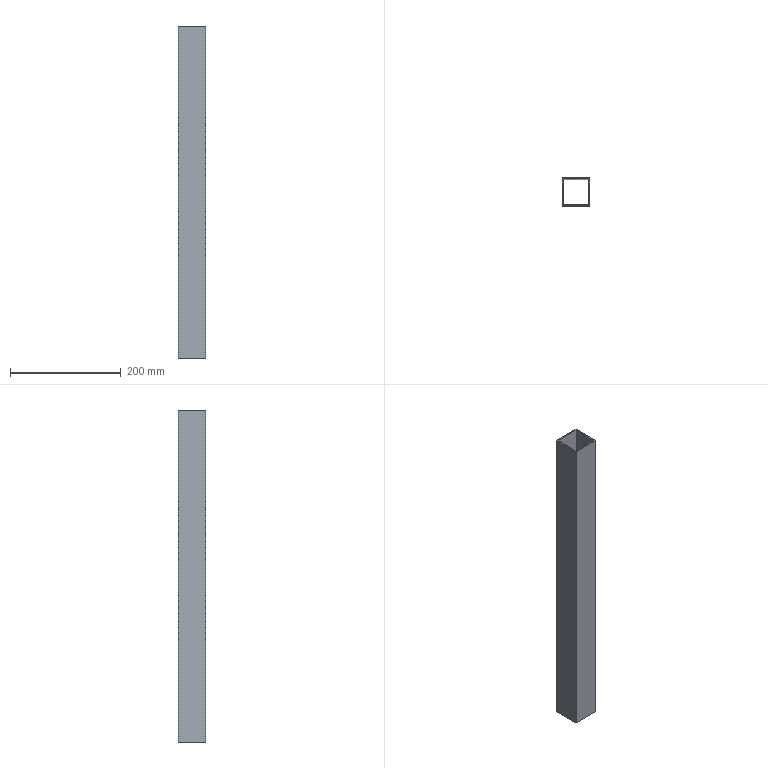Part | SolidWorks | features Extrusion 1 | 1 solid | 10 faces | box 50 x 50 x 600 mm | volume 230400 mm3 | plane 10
STEP:
#1=CARTESIAN_POINT('',(25.,-25.,600.));
#2=VERTEX_POINT('',#1);
#3=CARTESIAN_POINT('',(25.,25.,600.));
#4=VERTEX_POINT('',#3);
#5=CARTESIAN_POINT('',(25.,-25.,600.));
#6=DIRECTION('',(0.,1.,0.));
#7=VECTOR('',#6,1000.);
#8=LINE('',#5,#7);
#9=EDGE_CURVE('',#2,#4,#8,.T.);
#10=ORIENTED_EDGE('',*,*,#9,.T.);
#11=CARTESIAN_POINT('',(-25.,25.,600.));
#12=VERTEX_POINT('',#11);
#13=CARTESIAN_POINT('',(-25.,25.,600.));
#14=DIRECTION('',(-1.,0.,0.));
#15=VECTOR('',#14,1000.);
#16=LINE('',#13,#15);
#17=EDGE_CURVE('',#4,#12,#16,.T.);
#18=ORIENTED_EDGE('',*,*,#17,.T.);
#19=CARTESIAN_POINT('',(-25.,-25.,600.));
#20=VERTEX_POINT('',#19);
#21=CARTESIAN_POINT('',(-25.,-25.,600.));
#22=DIRECTION('',(0.,-1.,0.));
#23=VECTOR('',#22,1000.);
#24=LINE('',#21,#23);
#25=EDGE_CURVE('',#12,#20,#24,.T.);
#26=ORIENTED_EDGE('',*,*,#25,.T.);
#27=CARTESIAN_POINT('',(-25.,-25.,600.));
#28=DIRECTION('',(1.,0.,0.));
#29=VECTOR('',#28,1000.);
#30=LINE('',#27,#29);
#31=EDGE_CURVE('',#20,#2,#30,.T.);
#32=ORIENTED_EDGE('',*,*,#31,.T.);
#33=EDGE_LOOP('',(#10,#18,#26,#32));
#34=FACE_OUTER_BOUND('',#33,.T.);
#35=CARTESIAN_POINT('',(23.,-23.,600.));
#36=VERTEX_POINT('',#35);
#37=CARTESIAN_POINT('',(23.,23.,600.));
#38=VERTEX_POINT('',#37);
#39=CARTESIAN_POINT('',(23.,-23.,600.));
#40=DIRECTION('',(0.,1.,0.));
#41=VECTOR('',#40,1000.);
#42=LINE('',#39,#41);
#43=EDGE_CURVE('',#36,#38,#42,.T.);
#44=ORIENTED_EDGE('',*,*,#43,.F.);
#45=CARTESIAN_POINT('',(-23.,-23.,600.));
#46=VERTEX_POINT('',#45);
#47=CARTESIAN_POINT('',(-23.,-23.,600.));
#48=DIRECTION('',(1.,0.,0.));
#49=VECTOR('',#48,1000.);
#50=LINE('',#47,#49);
#51=EDGE_CURVE('',#46,#36,#50,.T.);
#52=ORIENTED_EDGE('',*,*,#51,.F.);
#53=CARTESIAN_POINT('',(-23.,23.,600.));
#54=VERTEX_POINT('',#53);
#55=CARTESIAN_POINT('',(-23.,-23.,600.));
#56=DIRECTION('',(0.,-1.,0.));
#57=VECTOR('',#56,1000.);
#58=LINE('',#55,#57);
#59=EDGE_CURVE('',#54,#46,#58,.T.);
#60=ORIENTED_EDGE('',*,*,#59,.F.);
#61=CARTESIAN_POINT('',(-23.,23.,600.));
#62=DIRECTION('',(-1.,0.,0.));
#63=VECTOR('',#62,1000.);
#64=LINE('',#61,#63);
#65=EDGE_CURVE('',#38,#54,#64,.T.);
#66=ORIENTED_EDGE('',*,*,#65,.F.);
#67=EDGE_LOOP('',(#44,#52,#60,#66));
#68=FACE_BOUND('',#67,.T.);
#69=CARTESIAN_POINT('',(0.,0.,600.));
#70=DIRECTION('',(0.,0.,-1.));
#71=DIRECTION('',(-1.,0.,0.));
#72=AXIS2_PLACEMENT_3D('',#69,#70,#71);
#73=PLANE('',#72);
#74=ADVANCED_FACE('',(#34,#68),#73,.F.);
#75=CARTESIAN_POINT('',(25.,-25.,0.));
#76=VERTEX_POINT('',#75);
#77=CARTESIAN_POINT('',(25.,25.,0.));
#78=VERTEX_POINT('',#77);
#79=CARTESIAN_POINT('',(25.,-25.,0.));
#80=DIRECTION('',(0.,1.,0.));
#81=VECTOR('',#80,1000.);
#82=LINE('',#79,#81);
#83=EDGE_CURVE('',#76,#78,#82,.T.);
#84=ORIENTED_EDGE('',*,*,#83,.F.);
#85=CARTESIAN_POINT('',(-25.,-25.,0.));
#86=VERTEX_POINT('',#85);
#87=CARTESIAN_POINT('',(-25.,-25.,0.));
#88=DIRECTION('',(1.,0.,0.));
#89=VECTOR('',#88,1000.);
#90=LINE('',#87,#89);
#91=EDGE_CURVE('',#86,#76,#90,.T.);
#92=ORIENTED_EDGE('',*,*,#91,.F.);
#93=CARTESIAN_POINT('',(-25.,25.,0.));
#94=VERTEX_POINT('',#93);
#95=CARTESIAN_POINT('',(-25.,-25.,0.));
#96=DIRECTION('',(0.,-1.,0.));
#97=VECTOR('',#96,1000.);
#98=LINE('',#95,#97);
#99=EDGE_CURVE('',#94,#86,#98,.T.);
#100=ORIENTED_EDGE('',*,*,#99,.F.);
#101=CARTESIAN_POINT('',(-25.,25.,0.));
#102=DIRECTION('',(-1.,0.,0.));
#103=VECTOR('',#102,1000.);
#104=LINE('',#101,#103);
#105=EDGE_CURVE('',#78,#94,#104,.T.);
#106=ORIENTED_EDGE('',*,*,#105,.F.);
#107=EDGE_LOOP('',(#84,#92,#100,#106));
#108=FACE_OUTER_BOUND('',#107,.T.);
#109=CARTESIAN_POINT('',(-23.,-23.,0.));
#110=VERTEX_POINT('',#109);
#111=CARTESIAN_POINT('',(23.,-23.,0.));
#112=VERTEX_POINT('',#111);
#113=CARTESIAN_POINT('',(-23.,-23.,0.));
#114=DIRECTION('',(1.,0.,0.));
#115=VECTOR('',#114,1000.);
#116=LINE('',#113,#115);
#117=EDGE_CURVE('',#110,#112,#116,.T.);
#118=ORIENTED_EDGE('',*,*,#117,.T.);
#119=CARTESIAN_POINT('',(23.,23.,0.));
#120=VERTEX_POINT('',#119);
#121=CARTESIAN_POINT('',(23.,-23.,0.));
#122=DIRECTION('',(0.,1.,0.));
#123=VECTOR('',#122,1000.);
#124=LINE('',#121,#123);
#125=EDGE_CURVE('',#112,#120,#124,.T.);
#126=ORIENTED_EDGE('',*,*,#125,.T.);
#127=CARTESIAN_POINT('',(-23.,23.,0.));
#128=VERTEX_POINT('',#127);
#129=CARTESIAN_POINT('',(-23.,23.,0.));
#130=DIRECTION('',(-1.,0.,0.));
#131=VECTOR('',#130,1000.);
#132=LINE('',#129,#131);
#133=EDGE_CURVE('',#120,#128,#132,.T.);
#134=ORIENTED_EDGE('',*,*,#133,.T.);
#135=CARTESIAN_POINT('',(-23.,-23.,0.));
#136=DIRECTION('',(0.,-1.,0.));
#137=VECTOR('',#136,1000.);
#138=LINE('',#135,#137);
#139=EDGE_CURVE('',#128,#110,#138,.T.);
#140=ORIENTED_EDGE('',*,*,#139,.T.);
#141=EDGE_LOOP('',(#118,#126,#134,#140));
#142=FACE_BOUND('',#141,.T.);
#143=CARTESIAN_POINT('',(0.,0.,0.));
#144=DIRECTION('',(0.,0.,-1.));
#145=DIRECTION('',(-1.,0.,0.));
#146=AXIS2_PLACEMENT_3D('',#143,#144,#145);
#147=PLANE('',#146);
#148=ADVANCED_FACE('',(#108,#142),#147,.T.);
#149=ORIENTED_EDGE('',*,*,#83,.T.);
#150=CARTESIAN_POINT('',(25.,25.,600.));
#151=DIRECTION('',(0.,0.,-1.));
#152=VECTOR('',#151,1000.);
#153=LINE('',#150,#152);
#154=EDGE_CURVE('',#4,#78,#153,.T.);
#155=ORIENTED_EDGE('',*,*,#154,.F.);
#156=ORIENTED_EDGE('',*,*,#9,.F.);
#157=CARTESIAN_POINT('',(25.,-25.,600.));
#158=DIRECTION('',(0.,0.,-1.));
#159=VECTOR('',#158,1000.);
#160=LINE('',#157,#159);
#161=EDGE_CURVE('',#2,#76,#160,.T.);
#162=ORIENTED_EDGE('',*,*,#161,.T.);
#163=EDGE_LOOP('',(#149,#155,#156,#162));
#164=FACE_OUTER_BOUND('',#163,.T.);
#165=CARTESIAN_POINT('',(25.,-25.,600.));
#166=DIRECTION('',(-1.,0.,0.));
#167=DIRECTION('',(0.,0.,1.));
#168=AXIS2_PLACEMENT_3D('',#165,#166,#167);
#169=PLANE('',#168);
#170=ADVANCED_FACE('',(#164),#169,.F.);
#171=ORIENTED_EDGE('',*,*,#105,.T.);
#172=CARTESIAN_POINT('',(-25.,25.,600.));
#173=DIRECTION('',(0.,0.,-1.));
#174=VECTOR('',#173,1000.);
#175=LINE('',#172,#174);
#176=EDGE_CURVE('',#12,#94,#175,.T.);
#177=ORIENTED_EDGE('',*,*,#176,.F.);
#178=ORIENTED_EDGE('',*,*,#17,.F.);
#179=ORIENTED_EDGE('',*,*,#154,.T.);
#180=EDGE_LOOP('',(#171,#177,#178,#179));
#181=FACE_OUTER_BOUND('',#180,.T.);
#182=CARTESIAN_POINT('',(-25.,25.,600.));
#183=DIRECTION('',(0.,-1.,0.));
#184=DIRECTION('',(0.,0.,-1.));
#185=AXIS2_PLACEMENT_3D('',#182,#183,#184);
#186=PLANE('',#185);
#187=ADVANCED_FACE('',(#181),#186,.F.);
#188=ORIENTED_EDGE('',*,*,#99,.T.);
#189=CARTESIAN_POINT('',(-25.,-25.,600.));
#190=DIRECTION('',(0.,0.,-1.));
#191=VECTOR('',#190,1000.);
#192=LINE('',#189,#191);
#193=EDGE_CURVE('',#20,#86,#192,.T.);
#194=ORIENTED_EDGE('',*,*,#193,.F.);
#195=ORIENTED_EDGE('',*,*,#25,.F.);
#196=ORIENTED_EDGE('',*,*,#176,.T.);
#197=EDGE_LOOP('',(#188,#194,#195,#196));
#198=FACE_OUTER_BOUND('',#197,.T.);
#199=CARTESIAN_POINT('',(-25.,-25.,600.));
#200=DIRECTION('',(1.,0.,0.));
#201=DIRECTION('',(0.,0.,-1.));
#202=AXIS2_PLACEMENT_3D('',#199,#200,#201);
#203=PLANE('',#202);
#204=ADVANCED_FACE('',(#198),#203,.F.);
#205=ORIENTED_EDGE('',*,*,#91,.T.);
#206=ORIENTED_EDGE('',*,*,#161,.F.);
#207=ORIENTED_EDGE('',*,*,#31,.F.);
#208=ORIENTED_EDGE('',*,*,#193,.T.);
#209=EDGE_LOOP('',(#205,#206,#207,#208));
#210=FACE_OUTER_BOUND('',#209,.T.);
#211=CARTESIAN_POINT('',(-25.,-25.,600.));
#212=DIRECTION('',(0.,1.,0.));
#213=DIRECTION('',(0.,0.,1.));
#214=AXIS2_PLACEMENT_3D('',#211,#212,#213);
#215=PLANE('',#214);
#216=ADVANCED_FACE('',(#210),#215,.F.);
#217=ORIENTED_EDGE('',*,*,#125,.F.);
#218=CARTESIAN_POINT('',(23.,-23.,600.));
#219=DIRECTION('',(0.,0.,-1.));
#220=VECTOR('',#219,1000.);
#221=LINE('',#218,#220);
#222=EDGE_CURVE('',#36,#112,#221,.T.);
#223=ORIENTED_EDGE('',*,*,#222,.F.);
#224=ORIENTED_EDGE('',*,*,#43,.T.);
#225=CARTESIAN_POINT('',(23.,23.,600.));
#226=DIRECTION('',(0.,0.,-1.));
#227=VECTOR('',#226,1000.);
#228=LINE('',#225,#227);
#229=EDGE_CURVE('',#38,#120,#228,.T.);
#230=ORIENTED_EDGE('',*,*,#229,.T.);
#231=EDGE_LOOP('',(#217,#223,#224,#230));
#232=FACE_OUTER_BOUND('',#231,.T.);
#233=CARTESIAN_POINT('',(23.,-23.,600.));
#234=DIRECTION('',(-1.,0.,0.));
#235=DIRECTION('',(0.,0.,1.));
#236=AXIS2_PLACEMENT_3D('',#233,#234,#235);
#237=PLANE('',#236);
#238=ADVANCED_FACE('',(#232),#237,.T.);
#239=ORIENTED_EDGE('',*,*,#133,.F.);
#240=ORIENTED_EDGE('',*,*,#229,.F.);
#241=ORIENTED_EDGE('',*,*,#65,.T.);
#242=CARTESIAN_POINT('',(-23.,23.,600.));
#243=DIRECTION('',(0.,0.,-1.));
#244=VECTOR('',#243,1000.);
#245=LINE('',#242,#244);
#246=EDGE_CURVE('',#54,#128,#245,.T.);
#247=ORIENTED_EDGE('',*,*,#246,.T.);
#248=EDGE_LOOP('',(#239,#240,#241,#247));
#249=FACE_OUTER_BOUND('',#248,.T.);
#250=CARTESIAN_POINT('',(-23.,23.,600.));
#251=DIRECTION('',(0.,-1.,0.));
#252=DIRECTION('',(0.,0.,-1.));
#253=AXIS2_PLACEMENT_3D('',#250,#251,#252);
#254=PLANE('',#253);
#255=ADVANCED_FACE('',(#249),#254,.T.);
#256=ORIENTED_EDGE('',*,*,#139,.F.);
#257=ORIENTED_EDGE('',*,*,#246,.F.);
#258=ORIENTED_EDGE('',*,*,#59,.T.);
#259=CARTESIAN_POINT('',(-23.,-23.,600.));
#260=DIRECTION('',(0.,0.,-1.));
#261=VECTOR('',#260,1000.);
#262=LINE('',#259,#261);
#263=EDGE_CURVE('',#46,#110,#262,.T.);
#264=ORIENTED_EDGE('',*,*,#263,.T.);
#265=EDGE_LOOP('',(#256,#257,#258,#264));
#266=FACE_OUTER_BOUND('',#265,.T.);
#267=CARTESIAN_POINT('',(-23.,-23.,600.));
#268=DIRECTION('',(1.,0.,0.));
#269=DIRECTION('',(0.,0.,-1.));
#270=AXIS2_PLACEMENT_3D('',#267,#268,#269);
#271=PLANE('',#270);
#272=ADVANCED_FACE('',(#266),#271,.T.);
#273=ORIENTED_EDGE('',*,*,#117,.F.);
#274=ORIENTED_EDGE('',*,*,#263,.F.);
#275=ORIENTED_EDGE('',*,*,#51,.T.);
#276=ORIENTED_EDGE('',*,*,#222,.T.);
#277=EDGE_LOOP('',(#273,#274,#275,#276));
#278=FACE_OUTER_BOUND('',#277,.T.);
#279=CARTESIAN_POINT('',(-23.,-23.,600.));
#280=DIRECTION('',(0.,1.,0.));
#281=DIRECTION('',(0.,0.,1.));
#282=AXIS2_PLACEMENT_3D('',#279,#280,#281);
#283=PLANE('',#282);
#284=ADVANCED_FACE('',(#278),#283,.T.);
#285=CLOSED_SHELL('',(#74,#148,#170,#187,#204,#216,#238,#255,#272,#284));
#286=MANIFOLD_SOLID_BREP('',#285);
#287=CARTESIAN_POINT('',(0.,0.,0.));
#288=DIRECTION('',(0.,0.,1.));
#289=DIRECTION('',(1.,0.,0.));
#290=AXIS2_PLACEMENT_3D('',#287,#288,#289);
#291=(LENGTH_UNIT()NAMED_UNIT(*)SI_UNIT(.MILLI.,.METRE.));
#292=UNCERTAINTY_MEASURE_WITH_UNIT(LENGTH_MEASURE(0.00001),#291,'','');
#293=(NAMED_UNIT(*)PLANE_ANGLE_UNIT()SI_UNIT($,.RADIAN.));
#294=(NAMED_UNIT(*)SI_UNIT($,.STERADIAN.)SOLID_ANGLE_UNIT());
#295=(GEOMETRIC_REPRESENTATION_CONTEXT(3)GLOBAL_UNCERTAINTY_ASSIGNED_CONTEXT((#292))GLOBAL_UNIT_ASSIGNED_CONTEXT((#291,#293,#294))REPRESENTATION_CONTEXT('',''));
#296=ADVANCED_BREP_SHAPE_REPRESENTATION('',(#286,#290),#295);